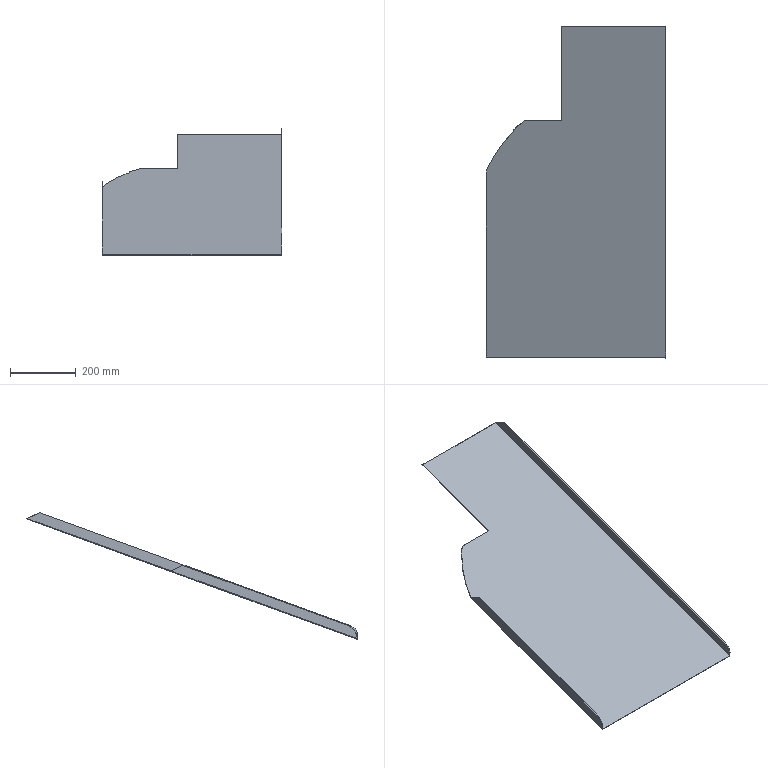Part | NX | features solid 2 | 1 solid | 17 faces | box 545 x 1007 x 384.916 mm | volume 1101359 mm3 | plane 13 | cylinder 2 | spline 2 | commonest cylinder face diameters 60 x1 90 x1
STEP:
#1=CARTESIAN_POINT('',(-203.,-1179.967,-588.65));
#2=VERTEX_POINT('',#1);
#3=CARTESIAN_POINT('',(-203.,-614.451,-382.819));
#4=VERTEX_POINT('',#3);
#5=CARTESIAN_POINT('',(-203.,-1653.904,-761.149));
#6=DIRECTION('',(0.,0.9397,0.342));
#7=VECTOR('',#6,1000.);
#8=LINE('',#5,#7);
#9=EDGE_CURVE('',#2,#4,#8,.T.);
#10=ORIENTED_EDGE('',*,*,#9,.F.);
#11=CARTESIAN_POINT('',(338.,-1179.967,-588.65));
#12=VERTEX_POINT('',#11);
#13=CARTESIAN_POINT('',(-203.,-1179.967,-588.65));
#14=DIRECTION('',(1.,0.,0.));
#15=VECTOR('',#14,1000.);
#16=LINE('',#13,#15);
#17=EDGE_CURVE('',#2,#12,#16,.T.);
#18=ORIENTED_EDGE('',*,*,#17,.T.);
#19=CARTESIAN_POINT('',(338.,-177.563,-223.805));
#20=VERTEX_POINT('',#19);
#21=CARTESIAN_POINT('',(338.,-1180.,-588.662));
#22=DIRECTION('',(0.,0.9397,0.342));
#23=VECTOR('',#22,1000.);
#24=LINE('',#21,#23);
#25=EDGE_CURVE('',#12,#20,#24,.T.);
#26=ORIENTED_EDGE('',*,*,#25,.T.);
#27=CARTESIAN_POINT('',(25.,-177.563,-223.805));
#28=VERTEX_POINT('',#27);
#29=CARTESIAN_POINT('',(620.,-177.563,-223.805));
#30=DIRECTION('',(-1.,0.,0.));
#31=VECTOR('',#30,1000.);
#32=LINE('',#29,#31);
#33=EDGE_CURVE('',#20,#28,#32,.T.);
#34=ORIENTED_EDGE('',*,*,#33,.T.);
#35=CARTESIAN_POINT('',(25.,-461.566,-327.173));
#36=VERTEX_POINT('',#35);
#37=CARTESIAN_POINT('',(25.,-1653.904,-761.149));
#38=DIRECTION('',(0.,-0.9397,-0.342));
#39=VECTOR('',#38,1000.);
#40=LINE('',#37,#39);
#41=EDGE_CURVE('',#28,#36,#40,.T.);
#42=ORIENTED_EDGE('',*,*,#41,.T.);
#43=CARTESIAN_POINT('',(-88.07,-461.566,-327.173));
#44=VERTEX_POINT('',#43);
#45=CARTESIAN_POINT('',(620.,-461.566,-327.173));
#46=DIRECTION('',(-1.,0.,0.));
#47=VECTOR('',#46,1000.);
#48=LINE('',#45,#47);
#49=EDGE_CURVE('',#44,#36,#48,.F.);
#50=ORIENTED_EDGE('',*,*,#49,.F.);
#51=CARTESIAN_POINT('',(-123.284,-495.559,-339.546));
#52=VERTEX_POINT('',#51);
#53=CARTESIAN_POINT('',(-88.07,-461.566,-327.173));
#54=CARTESIAN_POINT('',(-91.423,-464.038,-328.073));
#55=CARTESIAN_POINT('',(-98.033,-469.095,-329.914));
#56=CARTESIAN_POINT('',(-106.013,-475.744,-332.334));
#57=CARTESIAN_POINT('',(-111.4,-480.635,-334.114));
#58=CARTESIAN_POINT('',(-114.42,-483.489,-335.153));
#59=CARTESIAN_POINT('',(-116.682,-485.634,-335.933));
#60=CARTESIAN_POINT('',(-118.929,-487.788,-336.717));
#61=CARTESIAN_POINT('',(-121.32,-489.829,-337.46));
#62=CARTESIAN_POINT('',(-122.904,-492.524,-338.441));
#63=CARTESIAN_POINT('',(-123.25,-494.551,-339.179));
#64=CARTESIAN_POINT('',(-123.284,-495.559,-339.546));
#65=B_SPLINE_CURVE_WITH_KNOTS('',3,(#53,#54,#55,#56,#57,#58,#59,#60,#61,#62,#63,#64),.UNSPECIFIED.,.F.,.F.,(4,1,1,1,1,1,1,1,1,4),(0.0254,0.03818,0.05097,0.05736,0.06055,0.06375,0.06695,0.07014,0.07334,0.07653),.UNSPECIFIED.);
#66=EDGE_CURVE('',#44,#52,#65,.T.);
#67=ORIENTED_EDGE('',*,*,#66,.T.);
#68=CARTESIAN_POINT('',(-205.,-614.451,-382.819));
#69=VERTEX_POINT('',#68);
#70=CARTESIAN_POINT('',(-123.284,-495.559,-339.546));
#71=CARTESIAN_POINT('',(-125.444,-497.723,-340.333));
#72=CARTESIAN_POINT('',(-128.755,-500.917,-341.496));
#73=CARTESIAN_POINT('',(-132.797,-505.448,-343.145));
#74=CARTESIAN_POINT('',(-136.976,-509.88,-344.758));
#75=CARTESIAN_POINT('',(-142.024,-515.548,-346.821));
#76=CARTESIAN_POINT('',(-153.776,-529.412,-351.867));
#77=CARTESIAN_POINT('',(-166.397,-546.422,-358.058));
#78=CARTESIAN_POINT('',(-179.375,-566.79,-365.471));
#79=CARTESIAN_POINT('',(-188.374,-582.448,-371.171));
#80=CARTESIAN_POINT('',(-196.629,-598.48,-377.006));
#81=CARTESIAN_POINT('',(-202.218,-609.123,-380.88));
#82=CARTESIAN_POINT('',(-205.,-614.451,-382.819));
#83=B_SPLINE_CURVE_WITH_KNOTS('',3,(#70,#71,#72,#73,#74,#75,#76,#77,#78,#79,#80,#81,#82),.UNSPECIFIED.,.F.,.F.,(4,1,1,1,1,1,1,1,1,1,4),(0.,0.009432,0.01415,0.01886,0.0283,0.03773,0.07545,0.09432,0.1132,0.132,0.1509),.UNSPECIFIED.);
#84=EDGE_CURVE('',#52,#69,#83,.T.);
#85=ORIENTED_EDGE('',*,*,#84,.T.);
#86=CARTESIAN_POINT('',(620.,-614.451,-382.819));
#87=DIRECTION('',(-1.,0.,0.));
#88=VECTOR('',#87,1000.);
#89=LINE('',#86,#88);
#90=EDGE_CURVE('',#4,#69,#89,.T.);
#91=ORIENTED_EDGE('',*,*,#90,.F.);
#92=EDGE_LOOP('',(#10,#18,#26,#34,#42,#50,#67,#85,#91));
#93=FACE_BOUND('',#92,.T.);
#94=CARTESIAN_POINT('',(620.,-1653.904,-761.149));
#95=DIRECTION('',(0.,-0.342,0.9397));
#96=DIRECTION('',(1.,0.,0.));
#97=AXIS2_PLACEMENT_3D('',#94,#95,#96);
#98=PLANE('',#97);
#99=ADVANCED_FACE('',(#93),#98,.T.);
#100=CARTESIAN_POINT('',(25.,-460.882,-329.052));
#101=VERTEX_POINT('',#100);
#102=CARTESIAN_POINT('',(25.,-461.566,-327.173));
#103=DIRECTION('',(0.,0.342,-0.9397));
#104=VECTOR('',#103,1000.);
#105=LINE('',#102,#104);
#106=EDGE_CURVE('',#36,#101,#105,.T.);
#107=ORIENTED_EDGE('',*,*,#106,.F.);
#108=ORIENTED_EDGE('',*,*,#41,.F.);
#109=CARTESIAN_POINT('',(25.,-175.,-225.));
#110=VERTEX_POINT('',#109);
#111=CARTESIAN_POINT('',(25.,-155.47,-234.107));
#112=DIRECTION('',(0.,0.9063,-0.4226));
#113=VECTOR('',#112,1000.);
#114=LINE('',#111,#113);
#115=EDGE_CURVE('',#28,#110,#114,.T.);
#116=ORIENTED_EDGE('',*,*,#115,.T.);
#117=CARTESIAN_POINT('',(25.,-144.484,-213.893));
#118=DIRECTION('',(0.,-0.9397,-0.342));
#119=VECTOR('',#118,1000.);
#120=LINE('',#117,#119);
#121=EDGE_CURVE('',#101,#110,#120,.F.);
#122=ORIENTED_EDGE('',*,*,#121,.F.);
#123=EDGE_LOOP('',(#107,#108,#116,#122));
#124=FACE_BOUND('',#123,.T.);
#125=CARTESIAN_POINT('',(25.,-145.168,-212.014));
#126=DIRECTION('',(-1.,0.,0.));
#127=DIRECTION('',(0.,0.,1.));
#128=AXIS2_PLACEMENT_3D('',#125,#126,#127);
#129=PLANE('',#128);
#130=ADVANCED_FACE('',(#124),#129,.T.);
#131=CARTESIAN_POINT('',(340.,-1180.,-590.374));
#132=VERTEX_POINT('',#131);
#133=CARTESIAN_POINT('',(340.,-1180.,-590.79));
#134=VERTEX_POINT('',#133);
#135=CARTESIAN_POINT('',(340.,-1180.,-730.));
#136=DIRECTION('',(0.,0.,1.));
#137=VECTOR('',#136,1000.);
#138=LINE('',#135,#137);
#139=EDGE_CURVE('',#132,#134,#138,.F.);
#140=ORIENTED_EDGE('',*,*,#139,.F.);
#141=CARTESIAN_POINT('',(-205.,-1180.,-590.374));
#142=VERTEX_POINT('',#141);
#143=CARTESIAN_POINT('',(-625.,-1180.,-590.374));
#144=DIRECTION('',(-1.,0.,0.));
#145=VECTOR('',#144,1000.);
#146=LINE('',#143,#145);
#147=EDGE_CURVE('',#132,#142,#146,.T.);
#148=ORIENTED_EDGE('',*,*,#147,.T.);
#149=CARTESIAN_POINT('',(-205.,-1180.,-590.79));
#150=VERTEX_POINT('',#149);
#151=CARTESIAN_POINT('',(-205.,-1180.,-730.));
#152=DIRECTION('',(0.,0.,1.));
#153=VECTOR('',#152,1000.);
#154=LINE('',#151,#153);
#155=EDGE_CURVE('',#142,#150,#154,.F.);
#156=ORIENTED_EDGE('',*,*,#155,.T.);
#157=CARTESIAN_POINT('',(-625.,-1180.,-590.79));
#158=DIRECTION('',(1.,0.,0.));
#159=VECTOR('',#158,1000.);
#160=LINE('',#157,#159);
#161=EDGE_CURVE('',#134,#150,#160,.F.);
#162=ORIENTED_EDGE('',*,*,#161,.F.);
#163=EDGE_LOOP('',(#140,#148,#156,#162));
#164=FACE_BOUND('',#163,.T.);
#165=CARTESIAN_POINT('',(-625.,-1180.,-730.));
#166=DIRECTION('',(0.,1.,0.));
#167=DIRECTION('',(1.,0.,0.));
#168=AXIS2_PLACEMENT_3D('',#165,#166,#167);
#169=PLANE('',#168);
#170=ADVANCED_FACE('',(#164),#169,.F.);
#171=CARTESIAN_POINT('',(340.,-1162.07,-550.21));
#172=VERTEX_POINT('',#171);
#173=CARTESIAN_POINT('',(340.,-1179.97,-588.743));
#174=VERTEX_POINT('',#173);
#175=CARTESIAN_POINT('',(340.,-1151.809,-578.401));
#176=DIRECTION('',(1.,0.,0.));
#177=DIRECTION('',(0.,0.,-1.));
#178=AXIS2_PLACEMENT_3D('',#175,#176,#177);
#179=CIRCLE('',#178,30.);
#180=EDGE_CURVE('',#172,#174,#179,.T.);
#181=ORIENTED_EDGE('',*,*,#180,.T.);
#182=CARTESIAN_POINT('',(340.,-1135.,-590.374));
#183=DIRECTION('',(-1.,0.,0.));
#184=DIRECTION('',(0.,0.,1.));
#185=AXIS2_PLACEMENT_3D('',#182,#183,#184);
#186=CIRCLE('',#185,45.);
#187=EDGE_CURVE('',#174,#132,#186,.F.);
#188=ORIENTED_EDGE('',*,*,#187,.T.);
#189=ORIENTED_EDGE('',*,*,#139,.T.);
#190=CARTESIAN_POINT('',(340.,-175.,-225.));
#191=VERTEX_POINT('',#190);
#192=CARTESIAN_POINT('',(340.,-1653.22,-763.028));
#193=DIRECTION('',(0.,0.9397,0.342));
#194=VECTOR('',#193,1000.);
#195=LINE('',#192,#194);
#196=EDGE_CURVE('',#134,#191,#195,.T.);
#197=ORIENTED_EDGE('',*,*,#196,.T.);
#198=CARTESIAN_POINT('',(340.,-216.015,-205.874));
#199=VERTEX_POINT('',#198);
#200=CARTESIAN_POINT('',(340.,-175.,-225.));
#201=DIRECTION('',(0.,-0.9063,0.4226));
#202=VECTOR('',#201,1000.);
#203=LINE('',#200,#202);
#204=EDGE_CURVE('',#191,#199,#203,.T.);
#205=ORIENTED_EDGE('',*,*,#204,.T.);
#206=CARTESIAN_POINT('',(340.,-1190.261,-560.471));
#207=DIRECTION('',(0.,0.9397,0.342));
#208=VECTOR('',#207,1000.);
#209=LINE('',#206,#208);
#210=EDGE_CURVE('',#172,#199,#209,.T.);
#211=ORIENTED_EDGE('',*,*,#210,.F.);
#212=EDGE_LOOP('',(#181,#188,#189,#197,#205,#211));
#213=FACE_BOUND('',#212,.T.);
#214=CARTESIAN_POINT('',(340.,-1653.904,-761.149));
#215=DIRECTION('',(-1.,0.,0.));
#216=DIRECTION('',(0.,0.,1.));
#217=AXIS2_PLACEMENT_3D('',#214,#215,#216);
#218=PLANE('',#217);
#219=ADVANCED_FACE('',(#213),#218,.F.);
#220=CARTESIAN_POINT('',(-205.,-613.767,-384.698));
#221=VERTEX_POINT('',#220);
#222=CARTESIAN_POINT('',(-205.,-1653.22,-763.028));
#223=DIRECTION('',(0.,0.9397,0.342));
#224=VECTOR('',#223,1000.);
#225=LINE('',#222,#224);
#226=EDGE_CURVE('',#150,#221,#225,.T.);
#227=ORIENTED_EDGE('',*,*,#226,.T.);
#228=CARTESIAN_POINT('',(-123.284,-494.875,-341.425));
#229=VERTEX_POINT('',#228);
#230=CARTESIAN_POINT('',(-123.284,-494.875,-341.425));
#231=CARTESIAN_POINT('',(-125.444,-497.039,-342.213));
#232=CARTESIAN_POINT('',(-128.755,-500.233,-343.375));
#233=CARTESIAN_POINT('',(-132.797,-504.764,-345.024));
#234=CARTESIAN_POINT('',(-136.976,-509.196,-346.637));
#235=CARTESIAN_POINT('',(-142.024,-514.864,-348.7));
#236=CARTESIAN_POINT('',(-153.776,-528.728,-353.746));
#237=CARTESIAN_POINT('',(-166.397,-545.738,-359.938));
#238=CARTESIAN_POINT('',(-179.375,-566.106,-367.351));
#239=CARTESIAN_POINT('',(-188.374,-581.764,-373.05));
#240=CARTESIAN_POINT('',(-196.629,-597.796,-378.885));
#241=CARTESIAN_POINT('',(-202.218,-608.439,-382.759));
#242=CARTESIAN_POINT('',(-205.,-613.767,-384.698));
#243=B_SPLINE_CURVE_WITH_KNOTS('',3,(#230,#231,#232,#233,#234,#235,#236,#237,#238,#239,#240,#241,#242),.UNSPECIFIED.,.F.,.F.,(4,1,1,1,1,1,1,1,1,1,4),(0.,0.009432,0.01415,0.01886,0.0283,0.03773,0.07545,0.09432,0.1132,0.132,0.1509),.UNSPECIFIED.);
#244=EDGE_CURVE('',#229,#221,#243,.T.);
#245=ORIENTED_EDGE('',*,*,#244,.F.);
#246=CARTESIAN_POINT('',(-88.07,-460.882,-329.052));
#247=VERTEX_POINT('',#246);
#248=CARTESIAN_POINT('',(-88.07,-460.882,-329.052));
#249=CARTESIAN_POINT('',(-91.421,-463.352,-329.952));
#250=CARTESIAN_POINT('',(-98.022,-468.403,-331.79));
#251=CARTESIAN_POINT('',(-105.985,-475.037,-334.204));
#252=CARTESIAN_POINT('',(-111.355,-479.909,-335.978));
#253=CARTESIAN_POINT('',(-114.366,-482.754,-337.013));
#254=CARTESIAN_POINT('',(-116.62,-484.89,-337.791));
#255=CARTESIAN_POINT('',(-118.858,-487.045,-338.575));
#256=CARTESIAN_POINT('',(-121.235,-489.057,-339.307));
#257=CARTESIAN_POINT('',(-122.894,-491.779,-340.298));
#258=CARTESIAN_POINT('',(-123.249,-493.848,-341.051));
#259=CARTESIAN_POINT('',(-123.284,-494.875,-341.425));
#260=B_SPLINE_CURVE_WITH_KNOTS('',3,(#248,#249,#250,#251,#252,#253,#254,#255,#256,#257,#258,#259),.UNSPECIFIED.,.F.,.F.,(4,1,1,1,1,1,1,1,1,4),(0.1384,0.1512,0.164,0.1704,0.1735,0.1767,0.1799,0.1831,0.1863,0.1895),.UNSPECIFIED.);
#261=EDGE_CURVE('',#247,#229,#260,.T.);
#262=ORIENTED_EDGE('',*,*,#261,.F.);
#263=CARTESIAN_POINT('',(620.,-460.882,-329.052));
#264=DIRECTION('',(-1.,0.,0.));
#265=VECTOR('',#264,1000.);
#266=LINE('',#263,#265);
#267=EDGE_CURVE('',#247,#101,#266,.F.);
#268=ORIENTED_EDGE('',*,*,#267,.T.);
#269=ORIENTED_EDGE('',*,*,#121,.T.);
#270=CARTESIAN_POINT('',(-70.,-175.,-225.));
#271=DIRECTION('',(1.,0.,0.));
#272=VECTOR('',#271,1000.);
#273=LINE('',#270,#272);
#274=EDGE_CURVE('',#110,#191,#273,.T.);
#275=ORIENTED_EDGE('',*,*,#274,.T.);
#276=ORIENTED_EDGE('',*,*,#196,.F.);
#277=ORIENTED_EDGE('',*,*,#161,.T.);
#278=EDGE_LOOP('',(#227,#245,#262,#268,#269,#275,#276,#277));
#279=FACE_BOUND('',#278,.T.);
#280=CARTESIAN_POINT('',(620.,-1653.22,-763.028));
#281=DIRECTION('',(0.,-0.342,0.9397));
#282=DIRECTION('',(1.,0.,0.));
#283=AXIS2_PLACEMENT_3D('',#280,#281,#282);
#284=PLANE('',#283);
#285=ADVANCED_FACE('',(#279),#284,.F.);
#286=ORIENTED_EDGE('',*,*,#210,.T.);
#287=CARTESIAN_POINT('',(338.,-216.015,-205.874));
#288=VERTEX_POINT('',#287);
#289=CARTESIAN_POINT('',(-70.,-216.015,-205.874));
#290=DIRECTION('',(-1.,0.,0.));
#291=VECTOR('',#290,1000.);
#292=LINE('',#289,#291);
#293=EDGE_CURVE('',#199,#288,#292,.T.);
#294=ORIENTED_EDGE('',*,*,#293,.T.);
#295=CARTESIAN_POINT('',(338.,-1162.07,-550.21));
#296=VERTEX_POINT('',#295);
#297=CARTESIAN_POINT('',(338.,-1190.261,-560.471));
#298=DIRECTION('',(0.,0.9397,0.342));
#299=VECTOR('',#298,1000.);
#300=LINE('',#297,#299);
#301=EDGE_CURVE('',#296,#288,#300,.T.);
#302=ORIENTED_EDGE('',*,*,#301,.F.);
#303=CARTESIAN_POINT('',(340.,-1162.07,-550.21));
#304=DIRECTION('',(-1.,0.,0.));
#305=VECTOR('',#304,1000.);
#306=LINE('',#303,#305);
#307=EDGE_CURVE('',#296,#172,#306,.F.);
#308=ORIENTED_EDGE('',*,*,#307,.T.);
#309=EDGE_LOOP('',(#286,#294,#302,#308));
#310=FACE_BOUND('',#309,.T.);
#311=CARTESIAN_POINT('',(340.,-1190.261,-560.471));
#312=DIRECTION('',(0.,0.342,-0.9397));
#313=DIRECTION('',(0.,0.9397,0.342));
#314=AXIS2_PLACEMENT_3D('',#311,#312,#313);
#315=PLANE('',#314);
#316=ADVANCED_FACE('',(#310),#315,.F.);
#317=ORIENTED_EDGE('',*,*,#301,.T.);
#318=CARTESIAN_POINT('',(338.,-175.,-225.));
#319=DIRECTION('',(0.,0.9063,-0.4226));
#320=VECTOR('',#319,1000.);
#321=LINE('',#318,#320);
#322=EDGE_CURVE('',#288,#20,#321,.T.);
#323=ORIENTED_EDGE('',*,*,#322,.T.);
#324=ORIENTED_EDGE('',*,*,#25,.F.);
#325=CARTESIAN_POINT('',(338.,-1179.97,-588.743));
#326=VERTEX_POINT('',#325);
#327=CARTESIAN_POINT('',(338.,-1135.,-590.374));
#328=DIRECTION('',(1.,0.,0.));
#329=DIRECTION('',(0.,0.,-1.));
#330=AXIS2_PLACEMENT_3D('',#327,#328,#329);
#331=CIRCLE('',#330,45.);
#332=EDGE_CURVE('',#12,#326,#331,.T.);
#333=ORIENTED_EDGE('',*,*,#332,.T.);
#334=CARTESIAN_POINT('',(338.,-1151.809,-578.401));
#335=DIRECTION('',(1.,0.,0.));
#336=DIRECTION('',(0.,0.,-1.));
#337=AXIS2_PLACEMENT_3D('',#334,#335,#336);
#338=CIRCLE('',#337,30.);
#339=EDGE_CURVE('',#326,#296,#338,.F.);
#340=ORIENTED_EDGE('',*,*,#339,.T.);
#341=EDGE_LOOP('',(#317,#323,#324,#333,#340));
#342=FACE_BOUND('',#341,.T.);
#343=CARTESIAN_POINT('',(338.,-1180.,-588.662));
#344=DIRECTION('',(1.,0.,0.));
#345=DIRECTION('',(0.,0.,-1.));
#346=AXIS2_PLACEMENT_3D('',#343,#344,#345);
#347=PLANE('',#346);
#348=ADVANCED_FACE('',(#342),#347,.F.);
#349=ORIENTED_EDGE('',*,*,#180,.F.);
#350=ORIENTED_EDGE('',*,*,#307,.F.);
#351=ORIENTED_EDGE('',*,*,#339,.F.);
#352=CARTESIAN_POINT('',(338.,-1179.97,-588.743));
#353=DIRECTION('',(-1.,0.,0.));
#354=VECTOR('',#353,1000.);
#355=LINE('',#352,#354);
#356=EDGE_CURVE('',#326,#174,#355,.F.);
#357=ORIENTED_EDGE('',*,*,#356,.T.);
#358=EDGE_LOOP('',(#349,#350,#351,#357));
#359=FACE_BOUND('',#358,.T.);
#360=CARTESIAN_POINT('',(340.,-1151.809,-578.401));
#361=DIRECTION('',(-1.,0.,0.));
#362=DIRECTION('',(0.,0.,1.));
#363=AXIS2_PLACEMENT_3D('',#360,#361,#362);
#364=CYLINDRICAL_SURFACE('',#363,30.);
#365=ADVANCED_FACE('',(#359),#364,.T.);
#366=ORIENTED_EDGE('',*,*,#115,.F.);
#367=ORIENTED_EDGE('',*,*,#33,.F.);
#368=ORIENTED_EDGE('',*,*,#322,.F.);
#369=ORIENTED_EDGE('',*,*,#293,.F.);
#370=ORIENTED_EDGE('',*,*,#204,.F.);
#371=ORIENTED_EDGE('',*,*,#274,.F.);
#372=EDGE_LOOP('',(#366,#367,#368,#369,#370,#371));
#373=FACE_BOUND('',#372,.T.);
#374=CARTESIAN_POINT('',(-70.,-175.,-225.));
#375=DIRECTION('',(0.,0.4226,0.9063));
#376=DIRECTION('',(0.,-0.9063,0.4226));
#377=AXIS2_PLACEMENT_3D('',#374,#375,#376);
#378=PLANE('',#377);
#379=ADVANCED_FACE('',(#373),#378,.T.);
#380=ORIENTED_EDGE('',*,*,#244,.T.);
#381=CARTESIAN_POINT('',(-205.,-614.451,-382.819));
#382=CARTESIAN_POINT('',(-205.,-614.223,-383.445));
#383=CARTESIAN_POINT('',(-205.,-613.995,-384.072));
#384=CARTESIAN_POINT('',(-205.,-613.767,-384.698));
#385=B_SPLINE_CURVE_WITH_KNOTS('',3,(#381,#382,#383,#384),.UNSPECIFIED.,.F.,.F.,(4,4),(0.,1.),.UNSPECIFIED.);
#386=EDGE_CURVE('',#69,#221,#385,.T.);
#387=ORIENTED_EDGE('',*,*,#386,.F.);
#388=ORIENTED_EDGE('',*,*,#84,.F.);
#389=CARTESIAN_POINT('',(-123.284,-495.217,-340.485));
#390=DIRECTION('',(0.,0.342,-0.9397));
#391=VECTOR('',#390,1000.);
#392=LINE('',#389,#391);
#393=EDGE_CURVE('',#52,#229,#392,.T.);
#394=ORIENTED_EDGE('',*,*,#393,.T.);
#395=EDGE_LOOP('',(#380,#387,#388,#394));
#396=FACE_BOUND('',#395,.T.);
#397=CARTESIAN_POINT('',(-123.284,-495.559,-339.546));
#398=CARTESIAN_POINT('',(-123.284,-494.875,-341.425));
#399=CARTESIAN_POINT('',(-124.476,-496.753,-339.98));
#400=CARTESIAN_POINT('',(-124.476,-496.069,-341.86));
#401=CARTESIAN_POINT('',(-126.258,-498.54,-340.631));
#402=CARTESIAN_POINT('',(-126.258,-497.856,-342.51));
#403=CARTESIAN_POINT('',(-128.658,-500.937,-341.503));
#404=CARTESIAN_POINT('',(-128.658,-500.253,-343.382));
#405=CARTESIAN_POINT('',(-129.977,-502.321,-342.007));
#406=CARTESIAN_POINT('',(-129.977,-501.637,-343.886));
#407=CARTESIAN_POINT('',(-130.878,-503.312,-342.367));
#408=CARTESIAN_POINT('',(-130.878,-502.628,-344.247));
#409=CARTESIAN_POINT('',(-131.724,-504.248,-342.708));
#410=CARTESIAN_POINT('',(-131.724,-503.564,-344.588));
#411=CARTESIAN_POINT('',(-132.491,-505.085,-343.013));
#412=CARTESIAN_POINT('',(-132.491,-504.401,-344.892));
#413=CARTESIAN_POINT('',(-133.239,-505.896,-343.308));
#414=CARTESIAN_POINT('',(-133.239,-505.212,-345.187));
#415=CARTESIAN_POINT('',(-133.974,-506.682,-343.594));
#416=CARTESIAN_POINT('',(-133.974,-505.998,-345.473));
#417=CARTESIAN_POINT('',(-135.12,-507.912,-344.042));
#418=CARTESIAN_POINT('',(-135.12,-507.228,-345.921));
#419=CARTESIAN_POINT('',(-136.431,-509.333,-344.559));
#420=CARTESIAN_POINT('',(-136.431,-508.649,-346.438));
#421=CARTESIAN_POINT('',(-137.961,-511.013,-345.171));
#422=CARTESIAN_POINT('',(-137.961,-510.329,-347.05));
#423=CARTESIAN_POINT('',(-139.821,-513.085,-345.925));
#424=CARTESIAN_POINT('',(-139.821,-512.401,-347.804));
#425=CARTESIAN_POINT('',(-143.366,-517.122,-347.394));
#426=CARTESIAN_POINT('',(-143.366,-516.438,-349.273));
#427=CARTESIAN_POINT('',(-147.239,-521.706,-349.062));
#428=CARTESIAN_POINT('',(-147.239,-521.022,-350.942));
#429=CARTESIAN_POINT('',(-151.069,-526.423,-350.779));
#430=CARTESIAN_POINT('',(-151.069,-525.739,-352.658));
#431=CARTESIAN_POINT('',(-154.751,-531.076,-352.473));
#432=CARTESIAN_POINT('',(-154.751,-530.392,-354.352));
#433=CARTESIAN_POINT('',(-159.297,-537.045,-354.645));
#434=CARTESIAN_POINT('',(-159.297,-536.361,-356.525));
#435=CARTESIAN_POINT('',(-164.589,-544.359,-357.307));
#436=CARTESIAN_POINT('',(-164.589,-543.675,-359.187));
#437=CARTESIAN_POINT('',(-168.894,-550.623,-359.587));
#438=CARTESIAN_POINT('',(-168.894,-549.939,-361.466));
#439=CARTESIAN_POINT('',(-172.235,-555.676,-361.426));
#440=CARTESIAN_POINT('',(-172.235,-554.992,-363.306));
#441=CARTESIAN_POINT('',(-174.64,-559.407,-362.784));
#442=CARTESIAN_POINT('',(-174.64,-558.723,-364.664));
#443=CARTESIAN_POINT('',(-177.024,-563.2,-364.165));
#444=CARTESIAN_POINT('',(-177.024,-562.516,-366.044));
#445=CARTESIAN_POINT('',(-179.364,-567.021,-365.556));
#446=CARTESIAN_POINT('',(-179.364,-566.337,-367.435));
#447=CARTESIAN_POINT('',(-181.668,-570.88,-366.96));
#448=CARTESIAN_POINT('',(-181.668,-570.196,-368.84));
#449=CARTESIAN_POINT('',(-183.555,-574.126,-368.142));
#450=CARTESIAN_POINT('',(-183.555,-573.442,-370.021));
#451=CARTESIAN_POINT('',(-185.046,-576.74,-369.093));
#452=CARTESIAN_POINT('',(-185.046,-576.056,-370.972));
#453=CARTESIAN_POINT('',(-186.155,-578.71,-369.81));
#454=CARTESIAN_POINT('',(-186.155,-578.026,-371.689));
#455=CARTESIAN_POINT('',(-187.069,-580.357,-370.41));
#456=CARTESIAN_POINT('',(-187.069,-579.673,-372.289));
#457=CARTESIAN_POINT('',(-187.799,-581.684,-370.892));
#458=CARTESIAN_POINT('',(-187.799,-581.,-372.772));
#459=CARTESIAN_POINT('',(-188.248,-582.505,-371.191));
#460=CARTESIAN_POINT('',(-188.248,-581.821,-373.071));
#461=CARTESIAN_POINT('',(-188.618,-583.186,-371.439));
#462=CARTESIAN_POINT('',(-188.618,-582.502,-373.319));
#463=CARTESIAN_POINT('',(-188.82,-583.56,-371.575));
#464=CARTESIAN_POINT('',(-188.82,-582.876,-373.455));
#465=CARTESIAN_POINT('',(-189.046,-583.979,-371.728));
#466=CARTESIAN_POINT('',(-189.046,-583.295,-373.607));
#467=CARTESIAN_POINT('',(-189.037,-583.961,-371.721));
#468=CARTESIAN_POINT('',(-189.037,-583.276,-373.6));
#469=CARTESIAN_POINT('',(-189.12,-584.116,-371.778));
#470=CARTESIAN_POINT('',(-189.12,-583.432,-373.657));
#471=CARTESIAN_POINT('',(-189.208,-584.281,-371.838));
#472=CARTESIAN_POINT('',(-189.208,-583.597,-373.717));
#473=CARTESIAN_POINT('',(-189.414,-584.667,-371.978));
#474=CARTESIAN_POINT('',(-189.414,-583.983,-373.858));
#475=CARTESIAN_POINT('',(-189.732,-585.269,-372.197));
#476=CARTESIAN_POINT('',(-189.732,-584.585,-374.077));
#477=CARTESIAN_POINT('',(-190.396,-586.529,-372.656));
#478=CARTESIAN_POINT('',(-190.396,-585.845,-374.535));
#479=CARTESIAN_POINT('',(-191.506,-588.641,-373.425));
#480=CARTESIAN_POINT('',(-191.506,-587.957,-375.304));
#481=CARTESIAN_POINT('',(-193.883,-593.178,-375.076));
#482=CARTESIAN_POINT('',(-193.883,-592.494,-376.955));
#483=CARTESIAN_POINT('',(-197.981,-601.011,-377.927));
#484=CARTESIAN_POINT('',(-197.981,-600.327,-379.806));
#485=CARTESIAN_POINT('',(-202.46,-609.587,-381.048));
#486=CARTESIAN_POINT('',(-202.46,-608.902,-382.928));
#487=CARTESIAN_POINT('',(-205.,-614.451,-382.819));
#488=CARTESIAN_POINT('',(-205.,-613.767,-384.698));
#489=B_SPLINE_SURFACE_WITH_KNOTS('',3,1,((#397,#398),(#399,#400),(#401,#402),(#403,#404),(#405,#406),(#407,#408),(#409,#410),(#411,#412),(#413,#414),(#415,#416),(#417,#418),(#419,#420),(#421,#422),(#423,#424),(#425,#426),(#427,#428),(#429,#430),(#431,#432),(#433,#434),(#435,#436),(#437,#438),(#439,#440),(#441,#442),(#443,#444),(#445,#446),(#447,#448),(#449,#450),(#451,#452),(#453,#454),(#455,#456),(#457,#458),(#459,#460),(#461,#462),(#463,#464),(#465,#466),(#467,#468),(#469,#470),(#471,#472),(#473,#474),(#475,#476),(#477,#478),(#479,#480),(#481,#482),(#483,#484),(#485,#486),(#487,#488)),.SURF_OF_LINEAR_EXTRUSION.,.F.,.F.,.F.,(4,1,1,1,1,1,1,1,1,1,1,1,1,1,1,1,1,1,1,1,1,1,1,1,1,1,1,1,1,1,1,1,1,1,1,1,1,1,1,1,1,1,1,4),(2,2),(-0.04098,-0.008449,0.007817,0.02408,0.03221,0.04035,0.04848,0.05661,0.06475,0.07288,0.08914,0.1054,0.1217,0.1542,0.2193,0.2518,0.2843,0.3494,0.4144,0.4795,0.512,0.5446,0.5771,0.6096,0.6422,0.6747,0.691,0.7072,0.7235,0.7316,0.7398,0.7438,0.7479,0.7499,0.752,0.756,0.7642,0.7723,0.7886,0.8048,0.8373,0.8699,0.9349,1.),(0.,1.),.UNSPECIFIED.);
#490=ADVANCED_FACE('',(#396),#489,.F.);
#491=CARTESIAN_POINT('',(-205.,-1150.391,-548.088));
#492=VERTEX_POINT('',#491);
#493=CARTESIAN_POINT('',(-205.,-650.339,-366.084));
#494=VERTEX_POINT('',#493);
#495=CARTESIAN_POINT('',(-205.,-1190.261,-562.599));
#496=DIRECTION('',(0.,0.9397,0.342));
#497=VECTOR('',#496,1000.);
#498=LINE('',#495,#497);
#499=EDGE_CURVE('',#492,#494,#498,.T.);
#500=ORIENTED_EDGE('',*,*,#499,.T.);
#501=CARTESIAN_POINT('',(-205.,-1323.342,-52.257));
#502=DIRECTION('',(0.,0.9063,-0.4226));
#503=VECTOR('',#502,1000.);
#504=LINE('',#501,#503);
#505=EDGE_CURVE('',#494,#69,#504,.T.);
#506=ORIENTED_EDGE('',*,*,#505,.T.);
#507=ORIENTED_EDGE('',*,*,#386,.T.);
#508=ORIENTED_EDGE('',*,*,#226,.F.);
#509=ORIENTED_EDGE('',*,*,#155,.F.);
#510=CARTESIAN_POINT('',(-205.,-1135.,-590.374));
#511=DIRECTION('',(-1.,0.,0.));
#512=DIRECTION('',(0.,0.,1.));
#513=AXIS2_PLACEMENT_3D('',#510,#511,#512);
#514=CIRCLE('',#513,45.);
#515=EDGE_CURVE('',#142,#492,#514,.T.);
#516=ORIENTED_EDGE('',*,*,#515,.T.);
#517=EDGE_LOOP('',(#500,#506,#507,#508,#509,#516));
#518=FACE_BOUND('',#517,.T.);
#519=CARTESIAN_POINT('',(-205.,-1653.904,-761.149));
#520=DIRECTION('',(-1.,0.,0.));
#521=DIRECTION('',(0.,0.,1.));
#522=AXIS2_PLACEMENT_3D('',#519,#520,#521);
#523=PLANE('',#522);
#524=ADVANCED_FACE('',(#518),#523,.T.);
#525=ORIENTED_EDGE('',*,*,#267,.F.);
#526=CARTESIAN_POINT('',(-88.07,-461.566,-327.173));
#527=DIRECTION('',(0.,0.342,-0.9397));
#528=VECTOR('',#527,1000.);
#529=LINE('',#526,#528);
#530=EDGE_CURVE('',#44,#247,#529,.T.);
#531=ORIENTED_EDGE('',*,*,#530,.F.);
#532=ORIENTED_EDGE('',*,*,#49,.T.);
#533=ORIENTED_EDGE('',*,*,#106,.T.);
#534=EDGE_LOOP('',(#525,#531,#532,#533));
#535=FACE_BOUND('',#534,.T.);
#536=CARTESIAN_POINT('',(620.,-461.566,-327.173));
#537=DIRECTION('',(0.,0.9397,0.342));
#538=DIRECTION('',(0.,-0.342,0.9397));
#539=AXIS2_PLACEMENT_3D('',#536,#537,#538);
#540=PLANE('',#539);
#541=ADVANCED_FACE('',(#535),#540,.T.);
#542=ORIENTED_EDGE('',*,*,#66,.F.);
#543=ORIENTED_EDGE('',*,*,#530,.T.);
#544=ORIENTED_EDGE('',*,*,#261,.T.);
#545=ORIENTED_EDGE('',*,*,#393,.F.);
#546=EDGE_LOOP('',(#542,#543,#544,#545));
#547=FACE_BOUND('',#546,.T.);
#548=CARTESIAN_POINT('',(-88.07,-461.566,-327.173));
#549=CARTESIAN_POINT('',(-88.07,-460.882,-329.052));
#550=CARTESIAN_POINT('',(-88.957,-462.219,-327.411));
#551=CARTESIAN_POINT('',(-88.957,-461.535,-329.29));
#552=CARTESIAN_POINT('',(-90.679,-463.501,-327.878));
#553=CARTESIAN_POINT('',(-90.679,-462.817,-329.757));
#554=CARTESIAN_POINT('',(-94.413,-466.34,-328.911));
#555=CARTESIAN_POINT('',(-94.413,-465.656,-330.79));
#556=CARTESIAN_POINT('',(-98.844,-469.824,-330.179));
#557=CARTESIAN_POINT('',(-98.844,-469.14,-332.058));
#558=CARTESIAN_POINT('',(-103.001,-473.249,-331.425));
#559=CARTESIAN_POINT('',(-103.001,-472.565,-333.305));
#560=CARTESIAN_POINT('',(-106.171,-475.96,-332.412));
#561=CARTESIAN_POINT('',(-106.171,-475.276,-334.291));
#562=CARTESIAN_POINT('',(-108.227,-477.773,-333.072));
#563=CARTESIAN_POINT('',(-108.227,-477.089,-334.951));
#564=CARTESIAN_POINT('',(-109.89,-479.273,-333.618));
#565=CARTESIAN_POINT('',(-109.89,-478.589,-335.497));
#566=CARTESIAN_POINT('',(-110.911,-480.206,-333.958));
#567=CARTESIAN_POINT('',(-110.911,-479.522,-335.837));
#568=CARTESIAN_POINT('',(-111.683,-480.919,-334.217));
#569=CARTESIAN_POINT('',(-111.683,-480.235,-336.097));
#570=CARTESIAN_POINT('',(-112.041,-481.252,-334.338));
#571=CARTESIAN_POINT('',(-112.041,-480.568,-336.218));
#572=CARTESIAN_POINT('',(-112.344,-481.534,-334.441));
#573=CARTESIAN_POINT('',(-112.344,-480.85,-336.32));
#574=CARTESIAN_POINT('',(-112.787,-481.949,-334.592));
#575=CARTESIAN_POINT('',(-112.787,-481.265,-336.471));
#576=CARTESIAN_POINT('',(-113.37,-482.497,-334.791));
#577=CARTESIAN_POINT('',(-113.37,-481.813,-336.671));
#578=CARTESIAN_POINT('',(-114.008,-483.1,-335.011));
#579=CARTESIAN_POINT('',(-114.008,-482.416,-336.89));
#580=CARTESIAN_POINT('',(-114.614,-483.674,-335.22));
#581=CARTESIAN_POINT('',(-114.614,-482.99,-337.099));
#582=CARTESIAN_POINT('',(-115.075,-484.111,-335.379));
#583=CARTESIAN_POINT('',(-115.075,-483.427,-337.258));
#584=CARTESIAN_POINT('',(-115.752,-484.755,-335.613));
#585=CARTESIAN_POINT('',(-115.752,-484.071,-337.493));
#586=CARTESIAN_POINT('',(-116.52,-485.485,-335.879));
#587=CARTESIAN_POINT('',(-116.52,-484.801,-337.758));
#588=CARTESIAN_POINT('',(-117.272,-486.198,-336.138));
#589=CARTESIAN_POINT('',(-117.272,-485.514,-338.018));
#590=CARTESIAN_POINT('',(-117.87,-486.763,-336.344));
#591=CARTESIAN_POINT('',(-117.87,-486.079,-338.224));
#592=CARTESIAN_POINT('',(-118.228,-487.101,-336.467));
#593=CARTESIAN_POINT('',(-118.228,-486.417,-338.347));
#594=CARTESIAN_POINT('',(-118.458,-487.317,-336.546));
#595=CARTESIAN_POINT('',(-118.458,-486.633,-338.425));
#596=CARTESIAN_POINT('',(-118.547,-487.401,-336.576));
#597=CARTESIAN_POINT('',(-118.547,-486.717,-338.456));
#598=CARTESIAN_POINT('',(-118.802,-487.634,-336.661));
#599=CARTESIAN_POINT('',(-118.802,-486.95,-338.541));
#600=CARTESIAN_POINT('',(-119.089,-487.892,-336.755));
#601=CARTESIAN_POINT('',(-119.089,-487.208,-338.634));
#602=CARTESIAN_POINT('',(-119.327,-488.103,-336.832));
#603=CARTESIAN_POINT('',(-119.327,-487.419,-338.711));
#604=CARTESIAN_POINT('',(-119.507,-488.263,-336.89));
#605=CARTESIAN_POINT('',(-119.507,-487.579,-338.77));
#606=CARTESIAN_POINT('',(-119.623,-488.367,-336.928));
#607=CARTESIAN_POINT('',(-119.623,-487.683,-338.807));
#608=CARTESIAN_POINT('',(-119.81,-488.537,-336.99));
#609=CARTESIAN_POINT('',(-119.81,-487.853,-338.869));
#610=CARTESIAN_POINT('',(-120.02,-488.737,-337.063));
#611=CARTESIAN_POINT('',(-120.02,-488.053,-338.942));
#612=CARTESIAN_POINT('',(-120.165,-488.878,-337.114));
#613=CARTESIAN_POINT('',(-120.165,-488.194,-338.993));
#614=CARTESIAN_POINT('',(-120.527,-489.236,-337.244));
#615=CARTESIAN_POINT('',(-120.527,-488.552,-339.123));
#616=CARTESIAN_POINT('',(-120.914,-489.633,-337.389));
#617=CARTESIAN_POINT('',(-120.914,-488.949,-339.268));
#618=CARTESIAN_POINT('',(-121.24,-489.999,-337.522));
#619=CARTESIAN_POINT('',(-121.24,-489.315,-339.401));
#620=CARTESIAN_POINT('',(-121.335,-490.114,-337.564));
#621=CARTESIAN_POINT('',(-121.335,-489.43,-339.443));
#622=CARTESIAN_POINT('',(-121.603,-490.461,-337.69));
#623=CARTESIAN_POINT('',(-121.603,-489.777,-339.569));
#624=CARTESIAN_POINT('',(-121.851,-490.82,-337.821));
#625=CARTESIAN_POINT('',(-121.851,-490.135,-339.7));
#626=CARTESIAN_POINT('',(-122.236,-491.449,-338.05));
#627=CARTESIAN_POINT('',(-122.236,-490.765,-339.929));
#628=CARTESIAN_POINT('',(-122.622,-492.247,-338.34));
#629=CARTESIAN_POINT('',(-122.622,-491.563,-340.22));
#630=CARTESIAN_POINT('',(-123.088,-493.632,-338.844));
#631=CARTESIAN_POINT('',(-123.088,-492.948,-340.724));
#632=CARTESIAN_POINT('',(-123.257,-494.751,-339.252));
#633=CARTESIAN_POINT('',(-123.257,-494.067,-341.131));
#634=CARTESIAN_POINT('',(-123.284,-495.559,-339.546));
#635=CARTESIAN_POINT('',(-123.284,-494.875,-341.425));
#636=B_SPLINE_SURFACE_WITH_KNOTS('',3,1,((#548,#549),(#550,#551),(#552,#553),(#554,#555),(#556,#557),(#558,#559),(#560,#561),(#562,#563),(#564,#565),(#566,#567),(#568,#569),(#570,#571),(#572,#573),(#574,#575),(#576,#577),(#578,#579),(#580,#581),(#582,#583),(#584,#585),(#586,#587),(#588,#589),(#590,#591),(#592,#593),(#594,#595),(#596,#597),(#598,#599),(#600,#601),(#602,#603),(#604,#605),(#606,#607),(#608,#609),(#610,#611),(#612,#613),(#614,#615),(#616,#617),(#618,#619),(#620,#621),(#622,#623),(#624,#625),(#626,#627),(#628,#629),(#630,#631),(#632,#633),(#634,#635)),.SURF_OF_LINEAR_EXTRUSION.,.F.,.F.,.F.,(4,1,1,1,1,1,1,1,1,1,1,1,1,1,1,1,1,1,1,1,1,1,1,1,1,1,1,1,1,1,1,1,1,1,1,1,1,1,1,1,1,4),(2,2),(0.5971,0.6202,0.6434,0.6897,0.7359,0.7591,0.7822,0.7938,0.8053,0.8111,0.814,0.8169,0.8227,0.8285,0.8343,0.84,0.8429,0.8458,0.8516,0.8574,0.8632,0.869,0.8719,0.8747,0.8776,0.8805,0.882,0.8827,0.8834,0.8863,0.8892,0.8907,0.8921,0.8979,0.9037,0.9066,0.9094,0.9152,0.921,0.9326,0.9442,0.9673),(0.,1.),.UNSPECIFIED.);
#637=ADVANCED_FACE('',(#547),#636,.F.);
#638=CARTESIAN_POINT('',(-203.,-1150.391,-548.088));
#639=VERTEX_POINT('',#638);
#640=CARTESIAN_POINT('',(-203.,-650.339,-366.084));
#641=VERTEX_POINT('',#640);
#642=CARTESIAN_POINT('',(-203.,-1190.261,-562.599));
#643=DIRECTION('',(0.,0.9397,0.342));
#644=VECTOR('',#643,1000.);
#645=LINE('',#642,#644);
#646=EDGE_CURVE('',#639,#641,#645,.T.);
#647=ORIENTED_EDGE('',*,*,#646,.T.);
#648=CARTESIAN_POINT('',(-205.,-650.339,-366.084));
#649=DIRECTION('',(1.,0.,0.));
#650=VECTOR('',#649,1000.);
#651=LINE('',#648,#650);
#652=EDGE_CURVE('',#641,#494,#651,.F.);
#653=ORIENTED_EDGE('',*,*,#652,.T.);
#654=ORIENTED_EDGE('',*,*,#499,.F.);
#655=CARTESIAN_POINT('',(-205.,-1150.391,-548.088));
#656=DIRECTION('',(-1.,0.,0.));
#657=VECTOR('',#656,1000.);
#658=LINE('',#655,#657);
#659=EDGE_CURVE('',#492,#639,#658,.F.);
#660=ORIENTED_EDGE('',*,*,#659,.T.);
#661=EDGE_LOOP('',(#647,#653,#654,#660));
#662=FACE_BOUND('',#661,.T.);
#663=CARTESIAN_POINT('',(-205.,-1190.261,-562.599));
#664=DIRECTION('',(0.,0.342,-0.9397));
#665=DIRECTION('',(0.,0.9397,0.342));
#666=AXIS2_PLACEMENT_3D('',#663,#664,#665);
#667=PLANE('',#666);
#668=ADVANCED_FACE('',(#662),#667,.F.);
#669=ORIENTED_EDGE('',*,*,#9,.T.);
#670=CARTESIAN_POINT('',(-203.,-999.332,-203.346));
#671=DIRECTION('',(0.,-0.9063,0.4226));
#672=VECTOR('',#671,1000.);
#673=LINE('',#670,#672);
#674=EDGE_CURVE('',#4,#641,#673,.T.);
#675=ORIENTED_EDGE('',*,*,#674,.T.);
#676=ORIENTED_EDGE('',*,*,#646,.F.);
#677=CARTESIAN_POINT('',(-203.,-1135.,-590.374));
#678=DIRECTION('',(1.,0.,0.));
#679=DIRECTION('',(0.,0.,-1.));
#680=AXIS2_PLACEMENT_3D('',#677,#678,#679);
#681=CIRCLE('',#680,45.);
#682=EDGE_CURVE('',#639,#2,#681,.T.);
#683=ORIENTED_EDGE('',*,*,#682,.T.);
#684=EDGE_LOOP('',(#669,#675,#676,#683));
#685=FACE_BOUND('',#684,.T.);
#686=CARTESIAN_POINT('',(-203.,-1180.,-590.79));
#687=DIRECTION('',(1.,0.,0.));
#688=DIRECTION('',(0.,0.,-1.));
#689=AXIS2_PLACEMENT_3D('',#686,#687,#688);
#690=PLANE('',#689);
#691=ADVANCED_FACE('',(#685),#690,.T.);
#692=ORIENTED_EDGE('',*,*,#515,.F.);
#693=ORIENTED_EDGE('',*,*,#147,.F.);
#694=ORIENTED_EDGE('',*,*,#187,.F.);
#695=ORIENTED_EDGE('',*,*,#356,.F.);
#696=ORIENTED_EDGE('',*,*,#332,.F.);
#697=ORIENTED_EDGE('',*,*,#17,.F.);
#698=ORIENTED_EDGE('',*,*,#682,.F.);
#699=ORIENTED_EDGE('',*,*,#659,.F.);
#700=EDGE_LOOP('',(#692,#693,#694,#695,#696,#697,#698,#699));
#701=FACE_BOUND('',#700,.T.);
#702=CARTESIAN_POINT('',(-205.,-1135.,-590.374));
#703=DIRECTION('',(1.,0.,0.));
#704=DIRECTION('',(0.,0.,-1.));
#705=AXIS2_PLACEMENT_3D('',#702,#703,#704);
#706=CYLINDRICAL_SURFACE('',#705,45.);
#707=ADVANCED_FACE('',(#701),#706,.T.);
#708=ORIENTED_EDGE('',*,*,#505,.F.);
#709=ORIENTED_EDGE('',*,*,#652,.F.);
#710=ORIENTED_EDGE('',*,*,#674,.F.);
#711=ORIENTED_EDGE('',*,*,#90,.T.);
#712=EDGE_LOOP('',(#708,#709,#710,#711));
#713=FACE_BOUND('',#712,.T.);
#714=CARTESIAN_POINT('',(-205.,-614.451,-382.819));
#715=DIRECTION('',(0.,0.4226,0.9063));
#716=DIRECTION('',(0.,-0.9063,0.4226));
#717=AXIS2_PLACEMENT_3D('',#714,#715,#716);
#718=PLANE('',#717);
#719=ADVANCED_FACE('',(#713),#718,.T.);
#720=CLOSED_SHELL('',(#99,#130,#170,#219,#285,#316,#348,#365,#379,#490,#524,#541,#637,#668,#691,#707,#719));
#721=MANIFOLD_SOLID_BREP('',#720);
#722=(LENGTH_UNIT()NAMED_UNIT(*)SI_UNIT(.MILLI.,.METRE.));
#723=UNCERTAINTY_MEASURE_WITH_UNIT(LENGTH_MEASURE(0.0508),#722,'','');
#724=(NAMED_UNIT(*)PLANE_ANGLE_UNIT()SI_UNIT($,.RADIAN.));
#725=(NAMED_UNIT(*)SI_UNIT($,.STERADIAN.)SOLID_ANGLE_UNIT());
#726=(GEOMETRIC_REPRESENTATION_CONTEXT(3)GLOBAL_UNCERTAINTY_ASSIGNED_CONTEXT((#723))GLOBAL_UNIT_ASSIGNED_CONTEXT((#722,#724,#725))REPRESENTATION_CONTEXT('',''));
#727=ADVANCED_BREP_SHAPE_REPRESENTATION('',(#721),#726);